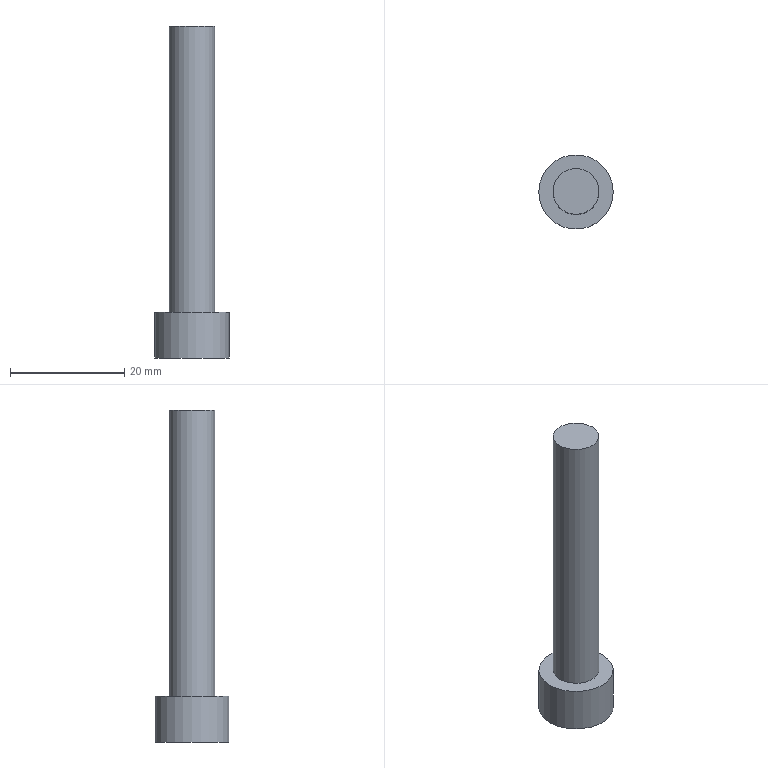Part | STEP file | 1 solid | 12 faces | box 13 x 13 x 58 mm | volume 3411 mm3 | plane 10 | cylinder 2 | commonest cylinder face diameters 8 x1 13 x1
STEP:
#1=CARTESIAN_POINT('',(0.,0.,0.));
#2=DIRECTION('',(0.,0.,1.));
#3=DIRECTION('',(1.,0.,0.));
#4=AXIS2_PLACEMENT_3D('',#1,#2,#3);
#5=CARTESIAN_POINT('',(1310.747,532.48,5.619));
#6=VERTEX_POINT('',#5);
#7=CARTESIAN_POINT('',(1317.247,532.48,5.619));
#8=DIRECTION('',(0.,0.,-1.));
#9=DIRECTION('',(-1.,0.,0.));
#10=AXIS2_PLACEMENT_3D('',#7,#8,#9);
#11=CIRCLE('',#10,6.5);
#12=CARTESIAN_POINT('',(1310.747,532.48,5.619));
#13=DIRECTION('',(0.,0.,1.));
#14=DIRECTION('',(1.,0.,0.));
#15=AXIS2_PLACEMENT_3D('',#12,#13,#14);
#16=PLANE('',#15);
#17=CARTESIAN_POINT('',(0.,0.));
#18=CARTESIAN_POINT('',(0.,11.258));
#19=CARTESIAN_POINT('',(9.75,5.629));
#20=CARTESIAN_POINT('',(19.5,0.));
#21=CARTESIAN_POINT('',(9.75,-5.629));
#22=CARTESIAN_POINT('',(0.,-11.258));
#23=CARTESIAN_POINT('',(0.,0.));
#24=(BOUNDED_CURVE()B_SPLINE_CURVE(2,(#17,#18,#19,#20,#21,#22,#23),.UNSPECIFIED.,.T.,.F.)B_SPLINE_CURVE_WITH_KNOTS((1,2,2,2,2,1),(-2.094,0.,2.094,4.189,6.283,8.378),.UNSPECIFIED.)CURVE()GEOMETRIC_REPRESENTATION_ITEM()RATIONAL_B_SPLINE_CURVE((1.,0.5,1.,0.5,1.,0.5,1.))REPRESENTATION_ITEM(''));
#25=(GEOMETRIC_REPRESENTATION_CONTEXT(2)PARAMETRIC_REPRESENTATION_CONTEXT()REPRESENTATION_CONTEXT('',''));
#26=DEFINITIONAL_REPRESENTATION('',(#24),#25);
#27=PCURVE('',#16,#26);
#28=CARTESIAN_POINT('',(1317.247,532.48,60.519));
#29=DIRECTION('',(0.,0.,-1.));
#30=DIRECTION('',(-1.,0.,0.));
#31=AXIS2_PLACEMENT_3D('',#28,#29,#30);
#32=CYLINDRICAL_SURFACE('',#31,6.5);
#33=CARTESIAN_POINT('',(0.,54.9));
#34=DIRECTION('',(1.,0.));
#35=VECTOR('',#34,1.);
#36=LINE('',#33,#35);
#37=(GEOMETRIC_REPRESENTATION_CONTEXT(2)PARAMETRIC_REPRESENTATION_CONTEXT()REPRESENTATION_CONTEXT('',''));
#38=DEFINITIONAL_REPRESENTATION('',(#36),#37);
#39=PCURVE('',#32,#38);
#40=SURFACE_CURVE('',#11,(#27,#39),.PCURVE_S1.);
#41=EDGE_CURVE('',#6,#6,#40,.T.);
#42=ORIENTED_EDGE('',*,*,#41,.T.);
#43=EDGE_LOOP('',(#42));
#44=FACE_BOUND('',#43,.T.);
#45=CARTESIAN_POINT('',(1318.979,535.48,5.619));
#46=VERTEX_POINT('',#45);
#47=CARTESIAN_POINT('',(1315.515,535.48,5.619));
#48=VERTEX_POINT('',#47);
#49=CARTESIAN_POINT('',(1318.979,535.48,5.619));
#50=DIRECTION('',(-1.,0.,0.));
#51=VECTOR('',#50,1.);
#52=LINE('',#49,#51);
#53=CARTESIAN_POINT('',(8.232,3.));
#54=DIRECTION('',(-1.,0.));
#55=VECTOR('',#54,1.);
#56=LINE('',#53,#55);
#57=(GEOMETRIC_REPRESENTATION_CONTEXT(2)PARAMETRIC_REPRESENTATION_CONTEXT()REPRESENTATION_CONTEXT('',''));
#58=DEFINITIONAL_REPRESENTATION('',(#56),#57);
#59=PCURVE('',#16,#58);
#60=CARTESIAN_POINT('',(1318.979,535.48,10.899));
#61=DIRECTION('',(0.,-1.,0.));
#62=DIRECTION('',(-1.,0.,0.));
#63=AXIS2_PLACEMENT_3D('',#60,#61,#62);
#64=PLANE('',#63);
#65=CARTESIAN_POINT('',(0.,5.28));
#66=DIRECTION('',(1.,0.));
#67=VECTOR('',#66,1.);
#68=LINE('',#65,#67);
#69=(GEOMETRIC_REPRESENTATION_CONTEXT(2)PARAMETRIC_REPRESENTATION_CONTEXT()REPRESENTATION_CONTEXT('',''));
#70=DEFINITIONAL_REPRESENTATION('',(#68),#69);
#71=PCURVE('',#64,#70);
#72=SURFACE_CURVE('',#52,(#59,#71),.PCURVE_S1.);
#73=EDGE_CURVE('',#46,#48,#72,.T.);
#74=ORIENTED_EDGE('',*,*,#73,.T.);
#75=CARTESIAN_POINT('',(1313.783,532.48,5.619));
#76=VERTEX_POINT('',#75);
#77=CARTESIAN_POINT('',(1315.515,535.48,5.619));
#78=DIRECTION('',(-0.5,-0.866,0.));
#79=VECTOR('',#78,1.);
#80=LINE('',#77,#79);
#81=CARTESIAN_POINT('',(4.768,3.));
#82=DIRECTION('',(-0.5,-0.866));
#83=VECTOR('',#82,1.);
#84=LINE('',#81,#83);
#85=(GEOMETRIC_REPRESENTATION_CONTEXT(2)PARAMETRIC_REPRESENTATION_CONTEXT()REPRESENTATION_CONTEXT('',''));
#86=DEFINITIONAL_REPRESENTATION('',(#84),#85);
#87=PCURVE('',#16,#86);
#88=CARTESIAN_POINT('',(1315.515,535.48,10.899));
#89=DIRECTION('',(0.866,-0.5,0.));
#90=DIRECTION('',(-0.5,-0.866,0.));
#91=AXIS2_PLACEMENT_3D('',#88,#89,#90);
#92=PLANE('',#91);
#93=CARTESIAN_POINT('',(0.,5.28));
#94=DIRECTION('',(1.,0.));
#95=VECTOR('',#94,1.);
#96=LINE('',#93,#95);
#97=(GEOMETRIC_REPRESENTATION_CONTEXT(2)PARAMETRIC_REPRESENTATION_CONTEXT()REPRESENTATION_CONTEXT('',''));
#98=DEFINITIONAL_REPRESENTATION('',(#96),#97);
#99=PCURVE('',#92,#98);
#100=SURFACE_CURVE('',#80,(#87,#99),.PCURVE_S1.);
#101=EDGE_CURVE('',#48,#76,#100,.T.);
#102=ORIENTED_EDGE('',*,*,#101,.T.);
#103=CARTESIAN_POINT('',(1315.515,529.48,5.619));
#104=VERTEX_POINT('',#103);
#105=CARTESIAN_POINT('',(1313.783,532.48,5.619));
#106=DIRECTION('',(0.5,-0.866,0.));
#107=VECTOR('',#106,1.);
#108=LINE('',#105,#107);
#109=CARTESIAN_POINT('',(3.036,0.));
#110=DIRECTION('',(0.5,-0.866));
#111=VECTOR('',#110,1.);
#112=LINE('',#109,#111);
#113=(GEOMETRIC_REPRESENTATION_CONTEXT(2)PARAMETRIC_REPRESENTATION_CONTEXT()REPRESENTATION_CONTEXT('',''));
#114=DEFINITIONAL_REPRESENTATION('',(#112),#113);
#115=PCURVE('',#16,#114);
#116=CARTESIAN_POINT('',(1313.783,532.48,10.899));
#117=DIRECTION('',(0.866,0.5,0.));
#118=DIRECTION('',(0.5,-0.866,0.));
#119=AXIS2_PLACEMENT_3D('',#116,#117,#118);
#120=PLANE('',#119);
#121=CARTESIAN_POINT('',(0.,5.28));
#122=DIRECTION('',(1.,0.));
#123=VECTOR('',#122,1.);
#124=LINE('',#121,#123);
#125=(GEOMETRIC_REPRESENTATION_CONTEXT(2)PARAMETRIC_REPRESENTATION_CONTEXT()REPRESENTATION_CONTEXT('',''));
#126=DEFINITIONAL_REPRESENTATION('',(#124),#125);
#127=PCURVE('',#120,#126);
#128=SURFACE_CURVE('',#108,(#115,#127),.PCURVE_S1.);
#129=EDGE_CURVE('',#76,#104,#128,.T.);
#130=ORIENTED_EDGE('',*,*,#129,.T.);
#131=CARTESIAN_POINT('',(1318.979,529.48,5.619));
#132=VERTEX_POINT('',#131);
#133=CARTESIAN_POINT('',(1315.515,529.48,5.619));
#134=DIRECTION('',(1.,0.,0.));
#135=VECTOR('',#134,1.);
#136=LINE('',#133,#135);
#137=CARTESIAN_POINT('',(4.768,-3.));
#138=DIRECTION('',(1.,0.));
#139=VECTOR('',#138,1.);
#140=LINE('',#137,#139);
#141=(GEOMETRIC_REPRESENTATION_CONTEXT(2)PARAMETRIC_REPRESENTATION_CONTEXT()REPRESENTATION_CONTEXT('',''));
#142=DEFINITIONAL_REPRESENTATION('',(#140),#141);
#143=PCURVE('',#16,#142);
#144=CARTESIAN_POINT('',(1315.515,529.48,10.899));
#145=DIRECTION('',(0.,1.,0.));
#146=DIRECTION('',(1.,0.,0.));
#147=AXIS2_PLACEMENT_3D('',#144,#145,#146);
#148=PLANE('',#147);
#149=CARTESIAN_POINT('',(0.,5.28));
#150=DIRECTION('',(1.,0.));
#151=VECTOR('',#150,1.);
#152=LINE('',#149,#151);
#153=(GEOMETRIC_REPRESENTATION_CONTEXT(2)PARAMETRIC_REPRESENTATION_CONTEXT()REPRESENTATION_CONTEXT('',''));
#154=DEFINITIONAL_REPRESENTATION('',(#152),#153);
#155=PCURVE('',#148,#154);
#156=SURFACE_CURVE('',#136,(#143,#155),.PCURVE_S1.);
#157=EDGE_CURVE('',#104,#132,#156,.T.);
#158=ORIENTED_EDGE('',*,*,#157,.T.);
#159=CARTESIAN_POINT('',(1320.711,532.48,5.619));
#160=VERTEX_POINT('',#159);
#161=CARTESIAN_POINT('',(1318.979,529.48,5.619));
#162=DIRECTION('',(0.5,0.866,0.));
#163=VECTOR('',#162,1.);
#164=LINE('',#161,#163);
#165=CARTESIAN_POINT('',(8.232,-3.));
#166=DIRECTION('',(0.5,0.866));
#167=VECTOR('',#166,1.);
#168=LINE('',#165,#167);
#169=(GEOMETRIC_REPRESENTATION_CONTEXT(2)PARAMETRIC_REPRESENTATION_CONTEXT()REPRESENTATION_CONTEXT('',''));
#170=DEFINITIONAL_REPRESENTATION('',(#168),#169);
#171=PCURVE('',#16,#170);
#172=CARTESIAN_POINT('',(1318.979,529.48,10.899));
#173=DIRECTION('',(-0.866,0.5,0.));
#174=DIRECTION('',(0.5,0.866,0.));
#175=AXIS2_PLACEMENT_3D('',#172,#173,#174);
#176=PLANE('',#175);
#177=CARTESIAN_POINT('',(0.,5.28));
#178=DIRECTION('',(1.,0.));
#179=VECTOR('',#178,1.);
#180=LINE('',#177,#179);
#181=(GEOMETRIC_REPRESENTATION_CONTEXT(2)PARAMETRIC_REPRESENTATION_CONTEXT()REPRESENTATION_CONTEXT('',''));
#182=DEFINITIONAL_REPRESENTATION('',(#180),#181);
#183=PCURVE('',#176,#182);
#184=SURFACE_CURVE('',#164,(#171,#183),.PCURVE_S1.);
#185=EDGE_CURVE('',#132,#160,#184,.T.);
#186=ORIENTED_EDGE('',*,*,#185,.T.);
#187=CARTESIAN_POINT('',(1320.711,532.48,5.619));
#188=DIRECTION('',(-0.5,0.866,0.));
#189=VECTOR('',#188,1.);
#190=LINE('',#187,#189);
#191=CARTESIAN_POINT('',(9.964,0.));
#192=DIRECTION('',(-0.5,0.866));
#193=VECTOR('',#192,1.);
#194=LINE('',#191,#193);
#195=(GEOMETRIC_REPRESENTATION_CONTEXT(2)PARAMETRIC_REPRESENTATION_CONTEXT()REPRESENTATION_CONTEXT('',''));
#196=DEFINITIONAL_REPRESENTATION('',(#194),#195);
#197=PCURVE('',#16,#196);
#198=CARTESIAN_POINT('',(1320.711,532.48,10.899));
#199=DIRECTION('',(-0.866,-0.5,0.));
#200=DIRECTION('',(-0.5,0.866,0.));
#201=AXIS2_PLACEMENT_3D('',#198,#199,#200);
#202=PLANE('',#201);
#203=CARTESIAN_POINT('',(0.,5.28));
#204=DIRECTION('',(1.,0.));
#205=VECTOR('',#204,1.);
#206=LINE('',#203,#205);
#207=(GEOMETRIC_REPRESENTATION_CONTEXT(2)PARAMETRIC_REPRESENTATION_CONTEXT()REPRESENTATION_CONTEXT('',''));
#208=DEFINITIONAL_REPRESENTATION('',(#206),#207);
#209=PCURVE('',#202,#208);
#210=SURFACE_CURVE('',#190,(#197,#209),.PCURVE_S1.);
#211=EDGE_CURVE('',#160,#46,#210,.T.);
#212=ORIENTED_EDGE('',*,*,#211,.T.);
#213=EDGE_LOOP('',(#74,#102,#130,#158,#186,#212));
#214=FACE_BOUND('',#213,.T.);
#215=ADVANCED_FACE('',(#44,#214),#16,.F.);
#216=ORIENTED_EDGE('',*,*,#41,.F.);
#217=CARTESIAN_POINT('',(1310.747,532.48,13.619));
#218=VERTEX_POINT('',#217);
#219=CARTESIAN_POINT('',(1310.747,532.48,13.619));
#220=CARTESIAN_POINT('',(1310.747,532.48,5.619));
#221=B_SPLINE_CURVE_WITH_KNOTS('',1,(#219,#220),.UNSPECIFIED.,.F.,.F.,(2,2),(46.9,54.9),.PIECEWISE_BEZIER_KNOTS.);
#222=CARTESIAN_POINT('',(0.,0.));
#223=DIRECTION('',(0.,1.));
#224=VECTOR('',#223,1.);
#225=LINE('',#222,#224);
#226=(GEOMETRIC_REPRESENTATION_CONTEXT(2)PARAMETRIC_REPRESENTATION_CONTEXT()REPRESENTATION_CONTEXT('',''));
#227=DEFINITIONAL_REPRESENTATION('',(#225),#226);
#228=PCURVE('',#32,#227);
#229=CARTESIAN_POINT('',(6.283,0.));
#230=DIRECTION('',(0.,1.));
#231=VECTOR('',#230,1.);
#232=LINE('',#229,#231);
#233=(GEOMETRIC_REPRESENTATION_CONTEXT(2)PARAMETRIC_REPRESENTATION_CONTEXT()REPRESENTATION_CONTEXT('',''));
#234=DEFINITIONAL_REPRESENTATION('',(#232),#233);
#235=PCURVE('',#32,#234);
#236=SEAM_CURVE('',#221,(#228,#235),.PCURVE_S1.);
#237=EDGE_CURVE('',#218,#6,#236,.T.);
#238=ORIENTED_EDGE('',*,*,#237,.F.);
#239=CARTESIAN_POINT('',(1317.247,532.48,13.619));
#240=DIRECTION('',(0.,0.,-1.));
#241=DIRECTION('',(-1.,0.,0.));
#242=AXIS2_PLACEMENT_3D('',#239,#240,#241);
#243=CIRCLE('',#242,6.5);
#244=CARTESIAN_POINT('',(0.,46.9));
#245=DIRECTION('',(1.,0.));
#246=VECTOR('',#245,1.);
#247=LINE('',#244,#246);
#248=(GEOMETRIC_REPRESENTATION_CONTEXT(2)PARAMETRIC_REPRESENTATION_CONTEXT()REPRESENTATION_CONTEXT('',''));
#249=DEFINITIONAL_REPRESENTATION('',(#247),#248);
#250=PCURVE('',#32,#249);
#251=CARTESIAN_POINT('',(1313.247,532.48,13.619));
#252=DIRECTION('',(0.,0.,-1.));
#253=DIRECTION('',(-1.,0.,0.));
#254=AXIS2_PLACEMENT_3D('',#251,#252,#253);
#255=PLANE('',#254);
#256=CARTESIAN_POINT('',(-4.,0.));
#257=DIRECTION('',(1.,0.));
#258=AXIS2_PLACEMENT_2D('',#256,#257);
#259=CIRCLE('',#258,6.5);
#260=(GEOMETRIC_REPRESENTATION_CONTEXT(2)PARAMETRIC_REPRESENTATION_CONTEXT()REPRESENTATION_CONTEXT('',''));
#261=DEFINITIONAL_REPRESENTATION('',(#259),#260);
#262=PCURVE('',#255,#261);
#263=SURFACE_CURVE('',#243,(#250,#262),.PCURVE_S1.);
#264=EDGE_CURVE('',#218,#218,#263,.T.);
#265=ORIENTED_EDGE('',*,*,#264,.T.);
#266=ORIENTED_EDGE('',*,*,#237,.T.);
#267=EDGE_LOOP('',(#216,#238,#265,#266));
#268=FACE_BOUND('',#267,.T.);
#269=ADVANCED_FACE('',(#268),#32,.T.);
#270=ORIENTED_EDGE('',*,*,#264,.F.);
#271=EDGE_LOOP('',(#270));
#272=FACE_BOUND('',#271,.T.);
#273=CARTESIAN_POINT('',(1313.247,532.48,13.619));
#274=VERTEX_POINT('',#273);
#275=CARTESIAN_POINT('',(1317.247,532.48,13.619));
#276=DIRECTION('',(0.,0.,-1.));
#277=DIRECTION('',(-1.,0.,0.));
#278=AXIS2_PLACEMENT_3D('',#275,#276,#277);
#279=CIRCLE('',#278,4.);
#280=CARTESIAN_POINT('',(-4.,0.));
#281=DIRECTION('',(1.,0.));
#282=AXIS2_PLACEMENT_2D('',#280,#281);
#283=CIRCLE('',#282,4.);
#284=(GEOMETRIC_REPRESENTATION_CONTEXT(2)PARAMETRIC_REPRESENTATION_CONTEXT()REPRESENTATION_CONTEXT('',''));
#285=DEFINITIONAL_REPRESENTATION('',(#283),#284);
#286=PCURVE('',#255,#285);
#287=CARTESIAN_POINT('',(1317.247,532.48,60.519));
#288=DIRECTION('',(0.,0.,-1.));
#289=DIRECTION('',(-1.,0.,0.));
#290=AXIS2_PLACEMENT_3D('',#287,#288,#289);
#291=CYLINDRICAL_SURFACE('',#290,4.);
#292=CARTESIAN_POINT('',(0.,46.9));
#293=DIRECTION('',(1.,0.));
#294=VECTOR('',#293,1.);
#295=LINE('',#292,#294);
#296=(GEOMETRIC_REPRESENTATION_CONTEXT(2)PARAMETRIC_REPRESENTATION_CONTEXT()REPRESENTATION_CONTEXT('',''));
#297=DEFINITIONAL_REPRESENTATION('',(#295),#296);
#298=PCURVE('',#291,#297);
#299=SURFACE_CURVE('',#279,(#286,#298),.PCURVE_S1.);
#300=EDGE_CURVE('',#274,#274,#299,.T.);
#301=ORIENTED_EDGE('',*,*,#300,.T.);
#302=EDGE_LOOP('',(#301));
#303=FACE_BOUND('',#302,.T.);
#304=ADVANCED_FACE('',(#272,#303),#255,.F.);
#305=ORIENTED_EDGE('',*,*,#300,.F.);
#306=CARTESIAN_POINT('',(1313.247,532.48,63.619));
#307=VERTEX_POINT('',#306);
#308=CARTESIAN_POINT('',(1313.247,532.48,63.619));
#309=CARTESIAN_POINT('',(1313.247,532.48,13.619));
#310=B_SPLINE_CURVE_WITH_KNOTS('',1,(#308,#309),.UNSPECIFIED.,.F.,.F.,(2,2),(-3.1,46.9),.PIECEWISE_BEZIER_KNOTS.);
#311=CARTESIAN_POINT('',(0.,0.));
#312=DIRECTION('',(0.,1.));
#313=VECTOR('',#312,1.);
#314=LINE('',#311,#313);
#315=(GEOMETRIC_REPRESENTATION_CONTEXT(2)PARAMETRIC_REPRESENTATION_CONTEXT()REPRESENTATION_CONTEXT('',''));
#316=DEFINITIONAL_REPRESENTATION('',(#314),#315);
#317=PCURVE('',#291,#316);
#318=CARTESIAN_POINT('',(6.283,0.));
#319=DIRECTION('',(0.,1.));
#320=VECTOR('',#319,1.);
#321=LINE('',#318,#320);
#322=(GEOMETRIC_REPRESENTATION_CONTEXT(2)PARAMETRIC_REPRESENTATION_CONTEXT()REPRESENTATION_CONTEXT('',''));
#323=DEFINITIONAL_REPRESENTATION('',(#321),#322);
#324=PCURVE('',#291,#323);
#325=SEAM_CURVE('',#310,(#317,#324),.PCURVE_S1.);
#326=EDGE_CURVE('',#307,#274,#325,.T.);
#327=ORIENTED_EDGE('',*,*,#326,.F.);
#328=CARTESIAN_POINT('',(1317.247,532.48,63.619));
#329=DIRECTION('',(0.,0.,-1.));
#330=DIRECTION('',(-1.,0.,0.));
#331=AXIS2_PLACEMENT_3D('',#328,#329,#330);
#332=CIRCLE('',#331,4.);
#333=CARTESIAN_POINT('',(0.,-3.1));
#334=DIRECTION('',(1.,0.));
#335=VECTOR('',#334,1.);
#336=LINE('',#333,#335);
#337=(GEOMETRIC_REPRESENTATION_CONTEXT(2)PARAMETRIC_REPRESENTATION_CONTEXT()REPRESENTATION_CONTEXT('',''));
#338=DEFINITIONAL_REPRESENTATION('',(#336),#337);
#339=PCURVE('',#291,#338);
#340=CARTESIAN_POINT('',(1317.247,532.48,63.619));
#341=DIRECTION('',(0.,0.,-1.));
#342=DIRECTION('',(-1.,0.,0.));
#343=AXIS2_PLACEMENT_3D('',#340,#341,#342);
#344=PLANE('',#343);
#345=CARTESIAN_POINT('',(0.,0.));
#346=DIRECTION('',(1.,0.));
#347=AXIS2_PLACEMENT_2D('',#345,#346);
#348=CIRCLE('',#347,4.);
#349=(GEOMETRIC_REPRESENTATION_CONTEXT(2)PARAMETRIC_REPRESENTATION_CONTEXT()REPRESENTATION_CONTEXT('',''));
#350=DEFINITIONAL_REPRESENTATION('',(#348),#349);
#351=PCURVE('',#344,#350);
#352=SURFACE_CURVE('',#332,(#339,#351),.PCURVE_S1.);
#353=EDGE_CURVE('',#307,#307,#352,.T.);
#354=ORIENTED_EDGE('',*,*,#353,.T.);
#355=ORIENTED_EDGE('',*,*,#326,.T.);
#356=EDGE_LOOP('',(#305,#327,#354,#355));
#357=FACE_BOUND('',#356,.T.);
#358=ADVANCED_FACE('',(#357),#291,.T.);
#359=ORIENTED_EDGE('',*,*,#353,.F.);
#360=EDGE_LOOP('',(#359));
#361=FACE_BOUND('',#360,.T.);
#362=ADVANCED_FACE('',(#361),#344,.F.);
#363=ORIENTED_EDGE('',*,*,#73,.F.);
#364=CARTESIAN_POINT('',(1318.979,535.48,10.899));
#365=VERTEX_POINT('',#364);
#366=CARTESIAN_POINT('',(1318.979,535.48,10.899));
#367=DIRECTION('',(0.,0.,1.));
#368=VECTOR('',#367,1.);
#369=LINE('',#366,#368);
#370=CARTESIAN_POINT('',(0.,0.));
#371=DIRECTION('',(0.,-1.));
#372=VECTOR('',#371,1.);
#373=LINE('',#370,#372);
#374=(GEOMETRIC_REPRESENTATION_CONTEXT(2)PARAMETRIC_REPRESENTATION_CONTEXT()REPRESENTATION_CONTEXT('',''));
#375=DEFINITIONAL_REPRESENTATION('',(#373),#374);
#376=PCURVE('',#64,#375);
#377=CARTESIAN_POINT('',(3.464,0.));
#378=DIRECTION('',(0.,-1.));
#379=VECTOR('',#378,1.);
#380=LINE('',#377,#379);
#381=(GEOMETRIC_REPRESENTATION_CONTEXT(2)PARAMETRIC_REPRESENTATION_CONTEXT()REPRESENTATION_CONTEXT('',''));
#382=DEFINITIONAL_REPRESENTATION('',(#380),#381);
#383=PCURVE('',#202,#382);
#384=SURFACE_CURVE('',#369,(#376,#383),.PCURVE_S1.);
#385=EDGE_CURVE('',#46,#365,#384,.T.);
#386=ORIENTED_EDGE('',*,*,#385,.T.);
#387=CARTESIAN_POINT('',(1315.515,535.48,10.899));
#388=VERTEX_POINT('',#387);
#389=CARTESIAN_POINT('',(1318.979,535.48,10.899));
#390=DIRECTION('',(1.,0.,0.));
#391=VECTOR('',#390,1.);
#392=LINE('',#389,#391);
#393=CARTESIAN_POINT('',(0.,0.));
#394=DIRECTION('',(-1.,0.));
#395=VECTOR('',#394,1.);
#396=LINE('',#393,#395);
#397=(GEOMETRIC_REPRESENTATION_CONTEXT(2)PARAMETRIC_REPRESENTATION_CONTEXT()REPRESENTATION_CONTEXT('',''));
#398=DEFINITIONAL_REPRESENTATION('',(#396),#397);
#399=PCURVE('',#64,#398);
#400=CARTESIAN_POINT('',(1317.247,532.48,10.899));
#401=DIRECTION('',(0.,0.,1.));
#402=DIRECTION('',(1.,0.,0.));
#403=AXIS2_PLACEMENT_3D('',#400,#401,#402);
#404=PLANE('',#403);
#405=CARTESIAN_POINT('',(1.732,3.));
#406=DIRECTION('',(1.,0.));
#407=VECTOR('',#406,1.);
#408=LINE('',#405,#407);
#409=(GEOMETRIC_REPRESENTATION_CONTEXT(2)PARAMETRIC_REPRESENTATION_CONTEXT()REPRESENTATION_CONTEXT('',''));
#410=DEFINITIONAL_REPRESENTATION('',(#408),#409);
#411=PCURVE('',#404,#410);
#412=SURFACE_CURVE('',#392,(#399,#411),.PCURVE_S1.);
#413=EDGE_CURVE('',#388,#365,#412,.T.);
#414=ORIENTED_EDGE('',*,*,#413,.F.);
#415=CARTESIAN_POINT('',(1315.515,535.48,10.899));
#416=DIRECTION('',(0.,0.,1.));
#417=VECTOR('',#416,1.);
#418=LINE('',#415,#417);
#419=CARTESIAN_POINT('',(3.464,0.));
#420=DIRECTION('',(0.,-1.));
#421=VECTOR('',#420,1.);
#422=LINE('',#419,#421);
#423=(GEOMETRIC_REPRESENTATION_CONTEXT(2)PARAMETRIC_REPRESENTATION_CONTEXT()REPRESENTATION_CONTEXT('',''));
#424=DEFINITIONAL_REPRESENTATION('',(#422),#423);
#425=PCURVE('',#64,#424);
#426=CARTESIAN_POINT('',(0.,0.));
#427=DIRECTION('',(0.,-1.));
#428=VECTOR('',#427,1.);
#429=LINE('',#426,#428);
#430=(GEOMETRIC_REPRESENTATION_CONTEXT(2)PARAMETRIC_REPRESENTATION_CONTEXT()REPRESENTATION_CONTEXT('',''));
#431=DEFINITIONAL_REPRESENTATION('',(#429),#430);
#432=PCURVE('',#92,#431);
#433=SURFACE_CURVE('',#418,(#425,#432),.PCURVE_S1.);
#434=EDGE_CURVE('',#48,#388,#433,.T.);
#435=ORIENTED_EDGE('',*,*,#434,.F.);
#436=EDGE_LOOP('',(#363,#386,#414,#435));
#437=FACE_BOUND('',#436,.T.);
#438=ADVANCED_FACE('',(#437),#64,.T.);
#439=ORIENTED_EDGE('',*,*,#101,.F.);
#440=ORIENTED_EDGE('',*,*,#434,.T.);
#441=CARTESIAN_POINT('',(1313.783,532.48,10.899));
#442=VERTEX_POINT('',#441);
#443=CARTESIAN_POINT('',(1315.515,535.48,10.899));
#444=DIRECTION('',(0.5,0.866,0.));
#445=VECTOR('',#444,1.);
#446=LINE('',#443,#445);
#447=CARTESIAN_POINT('',(0.,0.));
#448=DIRECTION('',(-1.,0.));
#449=VECTOR('',#448,1.);
#450=LINE('',#447,#449);
#451=(GEOMETRIC_REPRESENTATION_CONTEXT(2)PARAMETRIC_REPRESENTATION_CONTEXT()REPRESENTATION_CONTEXT('',''));
#452=DEFINITIONAL_REPRESENTATION('',(#450),#451);
#453=PCURVE('',#92,#452);
#454=CARTESIAN_POINT('',(-1.732,3.));
#455=DIRECTION('',(0.5,0.866));
#456=VECTOR('',#455,1.);
#457=LINE('',#454,#456);
#458=(GEOMETRIC_REPRESENTATION_CONTEXT(2)PARAMETRIC_REPRESENTATION_CONTEXT()REPRESENTATION_CONTEXT('',''));
#459=DEFINITIONAL_REPRESENTATION('',(#457),#458);
#460=PCURVE('',#404,#459);
#461=SURFACE_CURVE('',#446,(#453,#460),.PCURVE_S1.);
#462=EDGE_CURVE('',#442,#388,#461,.T.);
#463=ORIENTED_EDGE('',*,*,#462,.F.);
#464=CARTESIAN_POINT('',(1313.783,532.48,10.899));
#465=DIRECTION('',(0.,0.,1.));
#466=VECTOR('',#465,1.);
#467=LINE('',#464,#466);
#468=CARTESIAN_POINT('',(3.464,0.));
#469=DIRECTION('',(0.,-1.));
#470=VECTOR('',#469,1.);
#471=LINE('',#468,#470);
#472=(GEOMETRIC_REPRESENTATION_CONTEXT(2)PARAMETRIC_REPRESENTATION_CONTEXT()REPRESENTATION_CONTEXT('',''));
#473=DEFINITIONAL_REPRESENTATION('',(#471),#472);
#474=PCURVE('',#92,#473);
#475=CARTESIAN_POINT('',(0.,0.));
#476=DIRECTION('',(0.,-1.));
#477=VECTOR('',#476,1.);
#478=LINE('',#475,#477);
#479=(GEOMETRIC_REPRESENTATION_CONTEXT(2)PARAMETRIC_REPRESENTATION_CONTEXT()REPRESENTATION_CONTEXT('',''));
#480=DEFINITIONAL_REPRESENTATION('',(#478),#479);
#481=PCURVE('',#120,#480);
#482=SURFACE_CURVE('',#467,(#474,#481),.PCURVE_S1.);
#483=EDGE_CURVE('',#76,#442,#482,.T.);
#484=ORIENTED_EDGE('',*,*,#483,.F.);
#485=EDGE_LOOP('',(#439,#440,#463,#484));
#486=FACE_BOUND('',#485,.T.);
#487=ADVANCED_FACE('',(#486),#92,.T.);
#488=ORIENTED_EDGE('',*,*,#129,.F.);
#489=ORIENTED_EDGE('',*,*,#483,.T.);
#490=CARTESIAN_POINT('',(1315.515,529.48,10.899));
#491=VERTEX_POINT('',#490);
#492=CARTESIAN_POINT('',(1313.783,532.48,10.899));
#493=DIRECTION('',(-0.5,0.866,0.));
#494=VECTOR('',#493,1.);
#495=LINE('',#492,#494);
#496=CARTESIAN_POINT('',(0.,0.));
#497=DIRECTION('',(-1.,0.));
#498=VECTOR('',#497,1.);
#499=LINE('',#496,#498);
#500=(GEOMETRIC_REPRESENTATION_CONTEXT(2)PARAMETRIC_REPRESENTATION_CONTEXT()REPRESENTATION_CONTEXT('',''));
#501=DEFINITIONAL_REPRESENTATION('',(#499),#500);
#502=PCURVE('',#120,#501);
#503=CARTESIAN_POINT('',(-3.464,0.));
#504=DIRECTION('',(-0.5,0.866));
#505=VECTOR('',#504,1.);
#506=LINE('',#503,#505);
#507=(GEOMETRIC_REPRESENTATION_CONTEXT(2)PARAMETRIC_REPRESENTATION_CONTEXT()REPRESENTATION_CONTEXT('',''));
#508=DEFINITIONAL_REPRESENTATION('',(#506),#507);
#509=PCURVE('',#404,#508);
#510=SURFACE_CURVE('',#495,(#502,#509),.PCURVE_S1.);
#511=EDGE_CURVE('',#491,#442,#510,.T.);
#512=ORIENTED_EDGE('',*,*,#511,.F.);
#513=CARTESIAN_POINT('',(1315.515,529.48,10.899));
#514=DIRECTION('',(0.,0.,1.));
#515=VECTOR('',#514,1.);
#516=LINE('',#513,#515);
#517=CARTESIAN_POINT('',(3.464,0.));
#518=DIRECTION('',(0.,-1.));
#519=VECTOR('',#518,1.);
#520=LINE('',#517,#519);
#521=(GEOMETRIC_REPRESENTATION_CONTEXT(2)PARAMETRIC_REPRESENTATION_CONTEXT()REPRESENTATION_CONTEXT('',''));
#522=DEFINITIONAL_REPRESENTATION('',(#520),#521);
#523=PCURVE('',#120,#522);
#524=CARTESIAN_POINT('',(0.,0.));
#525=DIRECTION('',(0.,-1.));
#526=VECTOR('',#525,1.);
#527=LINE('',#524,#526);
#528=(GEOMETRIC_REPRESENTATION_CONTEXT(2)PARAMETRIC_REPRESENTATION_CONTEXT()REPRESENTATION_CONTEXT('',''));
#529=DEFINITIONAL_REPRESENTATION('',(#527),#528);
#530=PCURVE('',#148,#529);
#531=SURFACE_CURVE('',#516,(#523,#530),.PCURVE_S1.);
#532=EDGE_CURVE('',#104,#491,#531,.T.);
#533=ORIENTED_EDGE('',*,*,#532,.F.);
#534=EDGE_LOOP('',(#488,#489,#512,#533));
#535=FACE_BOUND('',#534,.T.);
#536=ADVANCED_FACE('',(#535),#120,.T.);
#537=ORIENTED_EDGE('',*,*,#157,.F.);
#538=ORIENTED_EDGE('',*,*,#532,.T.);
#539=CARTESIAN_POINT('',(1318.979,529.48,10.899));
#540=VERTEX_POINT('',#539);
#541=CARTESIAN_POINT('',(1315.515,529.48,10.899));
#542=DIRECTION('',(-1.,0.,0.));
#543=VECTOR('',#542,1.);
#544=LINE('',#541,#543);
#545=CARTESIAN_POINT('',(0.,0.));
#546=DIRECTION('',(-1.,0.));
#547=VECTOR('',#546,1.);
#548=LINE('',#545,#547);
#549=(GEOMETRIC_REPRESENTATION_CONTEXT(2)PARAMETRIC_REPRESENTATION_CONTEXT()REPRESENTATION_CONTEXT('',''));
#550=DEFINITIONAL_REPRESENTATION('',(#548),#549);
#551=PCURVE('',#148,#550);
#552=CARTESIAN_POINT('',(-1.732,-3.));
#553=DIRECTION('',(-1.,0.));
#554=VECTOR('',#553,1.);
#555=LINE('',#552,#554);
#556=(GEOMETRIC_REPRESENTATION_CONTEXT(2)PARAMETRIC_REPRESENTATION_CONTEXT()REPRESENTATION_CONTEXT('',''));
#557=DEFINITIONAL_REPRESENTATION('',(#555),#556);
#558=PCURVE('',#404,#557);
#559=SURFACE_CURVE('',#544,(#551,#558),.PCURVE_S1.);
#560=EDGE_CURVE('',#540,#491,#559,.T.);
#561=ORIENTED_EDGE('',*,*,#560,.F.);
#562=CARTESIAN_POINT('',(1318.979,529.48,10.899));
#563=DIRECTION('',(0.,0.,1.));
#564=VECTOR('',#563,1.);
#565=LINE('',#562,#564);
#566=CARTESIAN_POINT('',(3.464,0.));
#567=DIRECTION('',(0.,-1.));
#568=VECTOR('',#567,1.);
#569=LINE('',#566,#568);
#570=(GEOMETRIC_REPRESENTATION_CONTEXT(2)PARAMETRIC_REPRESENTATION_CONTEXT()REPRESENTATION_CONTEXT('',''));
#571=DEFINITIONAL_REPRESENTATION('',(#569),#570);
#572=PCURVE('',#148,#571);
#573=CARTESIAN_POINT('',(0.,0.));
#574=DIRECTION('',(0.,-1.));
#575=VECTOR('',#574,1.);
#576=LINE('',#573,#575);
#577=(GEOMETRIC_REPRESENTATION_CONTEXT(2)PARAMETRIC_REPRESENTATION_CONTEXT()REPRESENTATION_CONTEXT('',''));
#578=DEFINITIONAL_REPRESENTATION('',(#576),#577);
#579=PCURVE('',#176,#578);
#580=SURFACE_CURVE('',#565,(#572,#579),.PCURVE_S1.);
#581=EDGE_CURVE('',#132,#540,#580,.T.);
#582=ORIENTED_EDGE('',*,*,#581,.F.);
#583=EDGE_LOOP('',(#537,#538,#561,#582));
#584=FACE_BOUND('',#583,.T.);
#585=ADVANCED_FACE('',(#584),#148,.T.);
#586=ORIENTED_EDGE('',*,*,#185,.F.);
#587=ORIENTED_EDGE('',*,*,#581,.T.);
#588=CARTESIAN_POINT('',(1320.711,532.48,10.899));
#589=VERTEX_POINT('',#588);
#590=CARTESIAN_POINT('',(1318.979,529.48,10.899));
#591=DIRECTION('',(-0.5,-0.866,0.));
#592=VECTOR('',#591,1.);
#593=LINE('',#590,#592);
#594=CARTESIAN_POINT('',(0.,0.));
#595=DIRECTION('',(-1.,0.));
#596=VECTOR('',#595,1.);
#597=LINE('',#594,#596);
#598=(GEOMETRIC_REPRESENTATION_CONTEXT(2)PARAMETRIC_REPRESENTATION_CONTEXT()REPRESENTATION_CONTEXT('',''));
#599=DEFINITIONAL_REPRESENTATION('',(#597),#598);
#600=PCURVE('',#176,#599);
#601=CARTESIAN_POINT('',(1.732,-3.));
#602=DIRECTION('',(-0.5,-0.866));
#603=VECTOR('',#602,1.);
#604=LINE('',#601,#603);
#605=(GEOMETRIC_REPRESENTATION_CONTEXT(2)PARAMETRIC_REPRESENTATION_CONTEXT()REPRESENTATION_CONTEXT('',''));
#606=DEFINITIONAL_REPRESENTATION('',(#604),#605);
#607=PCURVE('',#404,#606);
#608=SURFACE_CURVE('',#593,(#600,#607),.PCURVE_S1.);
#609=EDGE_CURVE('',#589,#540,#608,.T.);
#610=ORIENTED_EDGE('',*,*,#609,.F.);
#611=CARTESIAN_POINT('',(1320.711,532.48,10.899));
#612=DIRECTION('',(0.,0.,1.));
#613=VECTOR('',#612,1.);
#614=LINE('',#611,#613);
#615=CARTESIAN_POINT('',(3.464,0.));
#616=DIRECTION('',(0.,-1.));
#617=VECTOR('',#616,1.);
#618=LINE('',#615,#617);
#619=(GEOMETRIC_REPRESENTATION_CONTEXT(2)PARAMETRIC_REPRESENTATION_CONTEXT()REPRESENTATION_CONTEXT('',''));
#620=DEFINITIONAL_REPRESENTATION('',(#618),#619);
#621=PCURVE('',#176,#620);
#622=CARTESIAN_POINT('',(0.,0.));
#623=DIRECTION('',(0.,-1.));
#624=VECTOR('',#623,1.);
#625=LINE('',#622,#624);
#626=(GEOMETRIC_REPRESENTATION_CONTEXT(2)PARAMETRIC_REPRESENTATION_CONTEXT()REPRESENTATION_CONTEXT('',''));
#627=DEFINITIONAL_REPRESENTATION('',(#625),#626);
#628=PCURVE('',#202,#627);
#629=SURFACE_CURVE('',#614,(#621,#628),.PCURVE_S1.);
#630=EDGE_CURVE('',#160,#589,#629,.T.);
#631=ORIENTED_EDGE('',*,*,#630,.F.);
#632=EDGE_LOOP('',(#586,#587,#610,#631));
#633=FACE_BOUND('',#632,.T.);
#634=ADVANCED_FACE('',(#633),#176,.T.);
#635=ORIENTED_EDGE('',*,*,#211,.F.);
#636=ORIENTED_EDGE('',*,*,#630,.T.);
#637=CARTESIAN_POINT('',(1320.711,532.48,10.899));
#638=DIRECTION('',(0.5,-0.866,0.));
#639=VECTOR('',#638,1.);
#640=LINE('',#637,#639);
#641=CARTESIAN_POINT('',(0.,0.));
#642=DIRECTION('',(-1.,0.));
#643=VECTOR('',#642,1.);
#644=LINE('',#641,#643);
#645=(GEOMETRIC_REPRESENTATION_CONTEXT(2)PARAMETRIC_REPRESENTATION_CONTEXT()REPRESENTATION_CONTEXT('',''));
#646=DEFINITIONAL_REPRESENTATION('',(#644),#645);
#647=PCURVE('',#202,#646);
#648=CARTESIAN_POINT('',(3.464,0.));
#649=DIRECTION('',(0.5,-0.866));
#650=VECTOR('',#649,1.);
#651=LINE('',#648,#650);
#652=(GEOMETRIC_REPRESENTATION_CONTEXT(2)PARAMETRIC_REPRESENTATION_CONTEXT()REPRESENTATION_CONTEXT('',''));
#653=DEFINITIONAL_REPRESENTATION('',(#651),#652);
#654=PCURVE('',#404,#653);
#655=SURFACE_CURVE('',#640,(#647,#654),.PCURVE_S1.);
#656=EDGE_CURVE('',#365,#589,#655,.T.);
#657=ORIENTED_EDGE('',*,*,#656,.F.);
#658=ORIENTED_EDGE('',*,*,#385,.F.);
#659=EDGE_LOOP('',(#635,#636,#657,#658));
#660=FACE_BOUND('',#659,.T.);
#661=ADVANCED_FACE('',(#660),#202,.T.);
#662=ORIENTED_EDGE('',*,*,#413,.T.);
#663=ORIENTED_EDGE('',*,*,#656,.T.);
#664=ORIENTED_EDGE('',*,*,#609,.T.);
#665=ORIENTED_EDGE('',*,*,#560,.T.);
#666=ORIENTED_EDGE('',*,*,#511,.T.);
#667=ORIENTED_EDGE('',*,*,#462,.T.);
#668=EDGE_LOOP('',(#662,#663,#664,#665,#666,#667));
#669=FACE_BOUND('',#668,.T.);
#670=ADVANCED_FACE('',(#669),#404,.F.);
#671=CLOSED_SHELL('',(#215,#269,#304,#358,#362,#438,#487,#536,#585,#634,#661,#670));
#672=MANIFOLD_SOLID_BREP('',#671);
#673=(LENGTH_UNIT()NAMED_UNIT(*)SI_UNIT(.MILLI.,.METRE.));
#674=UNCERTAINTY_MEASURE_WITH_UNIT(LENGTH_MEASURE(0.000002),#673,'','');
#675=(NAMED_UNIT(*)PLANE_ANGLE_UNIT()SI_UNIT($,.RADIAN.));
#676=(NAMED_UNIT(*)SI_UNIT($,.STERADIAN.)SOLID_ANGLE_UNIT());
#677=(GEOMETRIC_REPRESENTATION_CONTEXT(3)GLOBAL_UNCERTAINTY_ASSIGNED_CONTEXT((#674))GLOBAL_UNIT_ASSIGNED_CONTEXT((#673,#675,#676))REPRESENTATION_CONTEXT('',''));
#678=ADVANCED_BREP_SHAPE_REPRESENTATION('',(#4,#672),#677);